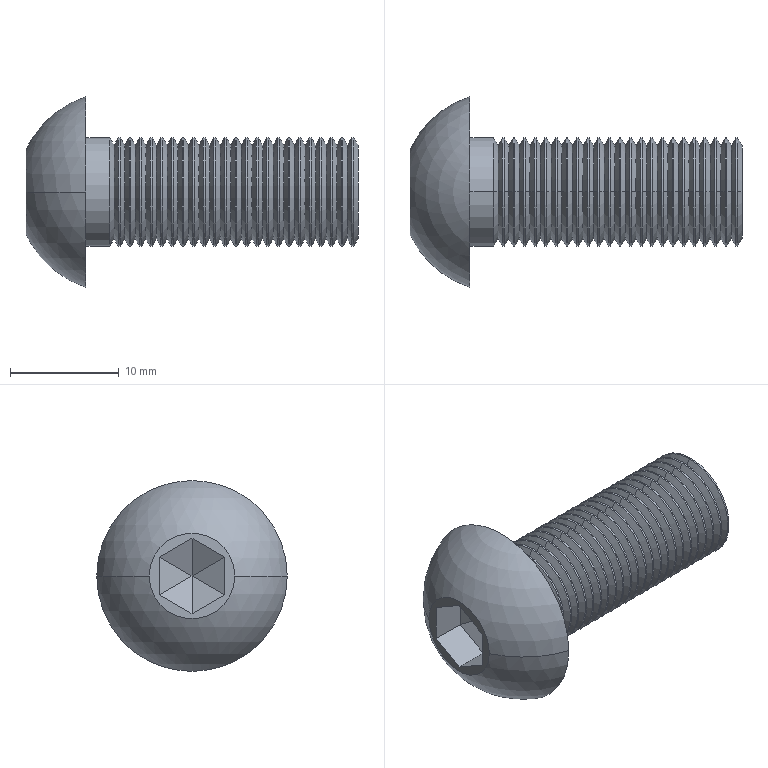Part | SolidWorks | features Cut 2, RevCut 2, Boss 1, Extrusion 1, Fillet 1, LPattern 1 | 1 solid | 159 faces | box 30.5 x 17.5 x 17.5 mm | volume 2529 mm3 | cone 94 | cylinder 48 | plane 15 | sphere 2 | commonest cylinder face diameters 10 x48